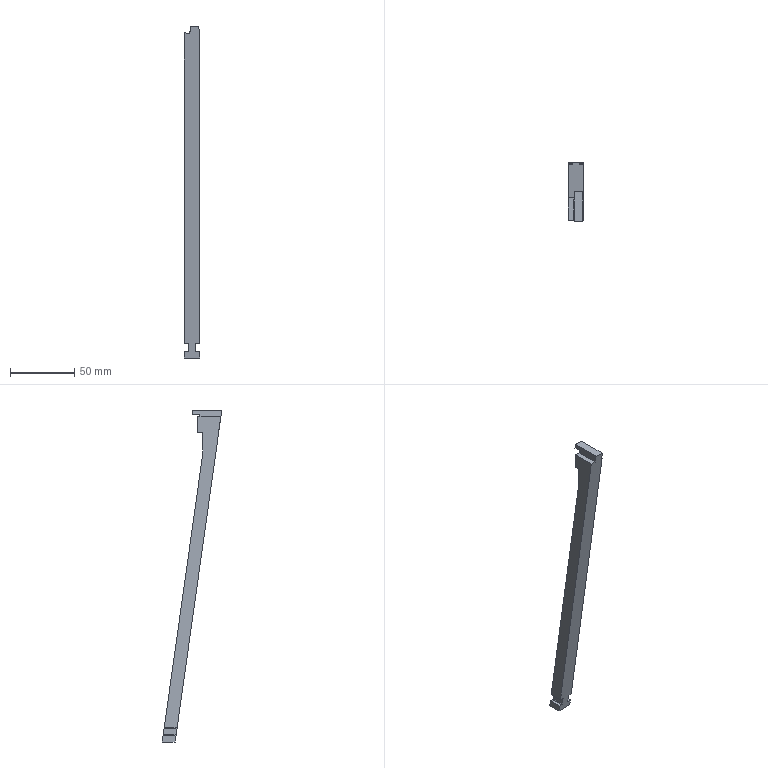Part | Creo | 1 solid | 95 faces | box 12 x 46.477 x 258.85 mm | volume 32281 mm3 | plane 48 | other 39 | cylinder 8 | commonest cylinder face diameters 1 x4 2 x1 7.151 x1 7.453 x1 28.412 x1